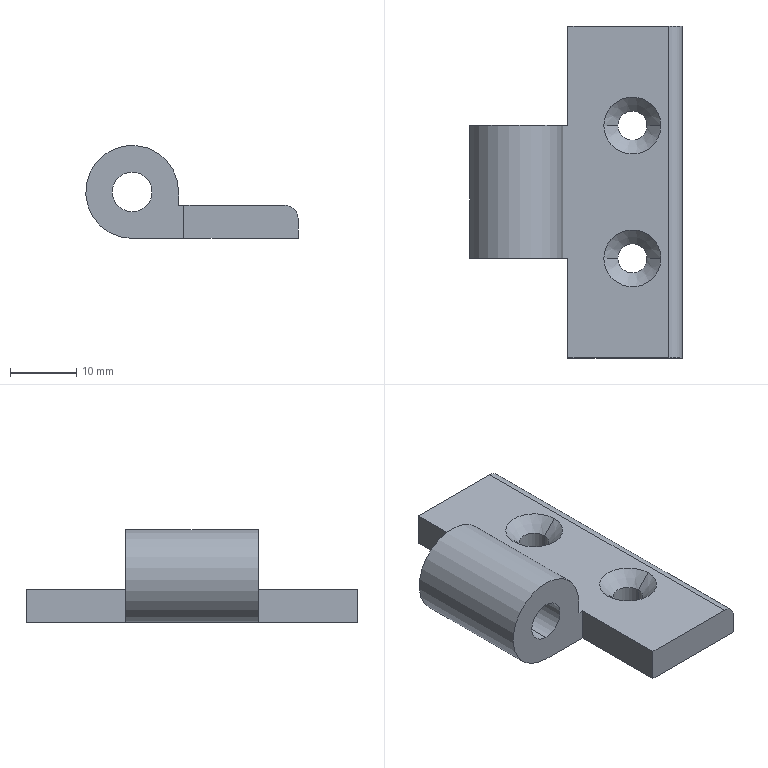Part | SolidWorks | features BaseBody 1 | 1 solid | 22 faces | box 32 x 50 x 14 mm | volume 6828 mm3 | plane 10 | cylinder 8 | cone 4 | commonest cylinder face diameters 4.4 x4 6 x2 4 x1 14 x1
STEP:
#1=CARTESIAN_POINT('',(0.,10.,4.));
#2=VERTEX_POINT('',#1);
#3=CARTESIAN_POINT('',(0.,10.,10.));
#4=VERTEX_POINT('',#3);
#5=CARTESIAN_POINT('',(0.,10.,7.));
#6=DIRECTION('',(0.,-1.,0.));
#7=DIRECTION('',(0.,0.,1.));
#8=AXIS2_PLACEMENT_3D('',#5,#6,#7);
#9=CIRCLE('',#8,3.);
#10=EDGE_CURVE('',#2,#4,#9,.T.);
#11=ORIENTED_EDGE('',*,*,#10,.F.);
#12=CARTESIAN_POINT('',(0.,-10.,4.));
#13=VERTEX_POINT('',#12);
#14=CARTESIAN_POINT('',(0.,23.,4.));
#15=DIRECTION('',(0.,-1.,0.));
#16=VECTOR('',#15,1000.);
#17=LINE('',#14,#16);
#18=EDGE_CURVE('',#2,#13,#17,.T.);
#19=ORIENTED_EDGE('',*,*,#18,.T.);
#20=CARTESIAN_POINT('',(0.,-10.,10.));
#21=VERTEX_POINT('',#20);
#22=CARTESIAN_POINT('',(0.,-10.,7.));
#23=DIRECTION('',(0.,1.,0.));
#24=DIRECTION('',(0.,0.,-1.));
#25=AXIS2_PLACEMENT_3D('',#22,#23,#24);
#26=CIRCLE('',#25,3.);
#27=EDGE_CURVE('',#21,#13,#26,.T.);
#28=ORIENTED_EDGE('',*,*,#27,.F.);
#29=CARTESIAN_POINT('',(0.,23.,10.));
#30=DIRECTION('',(0.,-1.,0.));
#31=VECTOR('',#30,1000.);
#32=LINE('',#29,#31);
#33=EDGE_CURVE('',#4,#21,#32,.T.);
#34=ORIENTED_EDGE('',*,*,#33,.F.);
#35=EDGE_LOOP('',(#11,#19,#28,#34));
#36=FACE_OUTER_BOUND('',#35,.T.);
#37=CARTESIAN_POINT('',(0.,23.,7.));
#38=DIRECTION('',(0.,-1.,0.));
#39=DIRECTION('',(0.,0.,1.));
#40=AXIS2_PLACEMENT_3D('',#37,#38,#39);
#41=CYLINDRICAL_SURFACE('',#40,3.);
#42=ADVANCED_FACE('',(#36),#41,.F.);
#43=CARTESIAN_POINT('',(15.3,-10.,0.));
#44=VERTEX_POINT('',#43);
#45=CARTESIAN_POINT('',(19.7,-10.,0.));
#46=VERTEX_POINT('',#45);
#47=CARTESIAN_POINT('',(17.5,-10.,0.));
#48=DIRECTION('',(0.,0.,-1.));
#49=DIRECTION('',(-1.,0.,0.));
#50=AXIS2_PLACEMENT_3D('',#47,#48,#49);
#51=CIRCLE('',#50,2.2);
#52=EDGE_CURVE('',#44,#46,#51,.T.);
#53=ORIENTED_EDGE('',*,*,#52,.T.);
#54=CARTESIAN_POINT('',(19.7,-10.,2.9));
#55=VERTEX_POINT('',#54);
#56=CARTESIAN_POINT('',(19.7,-10.,0.));
#57=DIRECTION('',(0.,0.,1.));
#58=VECTOR('',#57,1000.);
#59=LINE('',#56,#58);
#60=EDGE_CURVE('',#46,#55,#59,.T.);
#61=ORIENTED_EDGE('',*,*,#60,.T.);
#62=CARTESIAN_POINT('',(15.3,-10.,2.9));
#63=VERTEX_POINT('',#62);
#64=CARTESIAN_POINT('',(17.5,-10.,2.9));
#65=DIRECTION('',(0.,0.,-1.));
#66=DIRECTION('',(-1.,0.,0.));
#67=AXIS2_PLACEMENT_3D('',#64,#65,#66);
#68=CIRCLE('',#67,2.2);
#69=EDGE_CURVE('',#63,#55,#68,.T.);
#70=ORIENTED_EDGE('',*,*,#69,.F.);
#71=CARTESIAN_POINT('',(15.3,-10.,0.));
#72=DIRECTION('',(0.,0.,1.));
#73=VECTOR('',#72,1000.);
#74=LINE('',#71,#73);
#75=EDGE_CURVE('',#44,#63,#74,.T.);
#76=ORIENTED_EDGE('',*,*,#75,.F.);
#77=EDGE_LOOP('',(#53,#61,#70,#76));
#78=FACE_OUTER_BOUND('',#77,.T.);
#79=CARTESIAN_POINT('',(17.5,-10.,0.));
#80=DIRECTION('',(0.,0.,1.));
#81=DIRECTION('',(-1.,0.,0.));
#82=AXIS2_PLACEMENT_3D('',#79,#80,#81);
#83=CYLINDRICAL_SURFACE('',#82,2.2);
#84=ADVANCED_FACE('',(#78),#83,.F.);
#85=CARTESIAN_POINT('',(17.5,-10.,2.9));
#86=DIRECTION('',(0.,0.,-1.));
#87=DIRECTION('',(-1.,0.,0.));
#88=AXIS2_PLACEMENT_3D('',#85,#86,#87);
#89=CIRCLE('',#88,2.2);
#90=EDGE_CURVE('',#55,#63,#89,.T.);
#91=ORIENTED_EDGE('',*,*,#90,.T.);
#92=CARTESIAN_POINT('',(13.2,-10.,5.));
#93=VERTEX_POINT('',#92);
#94=CARTESIAN_POINT('',(13.2,-10.,5.));
#95=DIRECTION('',(-0.7071,0.,0.7071));
#96=VECTOR('',#95,1000.);
#97=LINE('',#94,#96);
#98=EDGE_CURVE('',#63,#93,#97,.T.);
#99=ORIENTED_EDGE('',*,*,#98,.T.);
#100=CARTESIAN_POINT('',(21.8,-10.,5.));
#101=VERTEX_POINT('',#100);
#102=CARTESIAN_POINT('',(17.5,-10.,5.));
#103=DIRECTION('',(0.,0.,-1.));
#104=DIRECTION('',(-1.,0.,0.));
#105=AXIS2_PLACEMENT_3D('',#102,#103,#104);
#106=CIRCLE('',#105,4.3);
#107=EDGE_CURVE('',#101,#93,#106,.T.);
#108=ORIENTED_EDGE('',*,*,#107,.F.);
#109=CARTESIAN_POINT('',(21.8,-10.,5.));
#110=DIRECTION('',(0.7071,0.,0.7071));
#111=VECTOR('',#110,1000.);
#112=LINE('',#109,#111);
#113=EDGE_CURVE('',#55,#101,#112,.T.);
#114=ORIENTED_EDGE('',*,*,#113,.F.);
#115=EDGE_LOOP('',(#91,#99,#108,#114));
#116=FACE_OUTER_BOUND('',#115,.T.);
#117=CARTESIAN_POINT('',(17.5,-10.,5.));
#118=DIRECTION('',(0.,0.,1.));
#119=DIRECTION('',(1.,0.,0.));
#120=AXIS2_PLACEMENT_3D('',#117,#118,#119);
#121=CONICAL_SURFACE('',#120,4.3,0.7854);
#122=ADVANCED_FACE('',(#116),#121,.F.);
#123=CARTESIAN_POINT('',(15.3,10.,0.));
#124=VERTEX_POINT('',#123);
#125=CARTESIAN_POINT('',(19.7,10.,0.));
#126=VERTEX_POINT('',#125);
#127=CARTESIAN_POINT('',(17.5,10.,0.));
#128=DIRECTION('',(0.,0.,-1.));
#129=DIRECTION('',(-1.,0.,0.));
#130=AXIS2_PLACEMENT_3D('',#127,#128,#129);
#131=CIRCLE('',#130,2.2);
#132=EDGE_CURVE('',#124,#126,#131,.T.);
#133=ORIENTED_EDGE('',*,*,#132,.T.);
#134=CARTESIAN_POINT('',(19.7,10.,2.9));
#135=VERTEX_POINT('',#134);
#136=CARTESIAN_POINT('',(19.7,10.,0.));
#137=DIRECTION('',(0.,0.,1.));
#138=VECTOR('',#137,1000.);
#139=LINE('',#136,#138);
#140=EDGE_CURVE('',#126,#135,#139,.T.);
#141=ORIENTED_EDGE('',*,*,#140,.T.);
#142=CARTESIAN_POINT('',(15.3,10.,2.9));
#143=VERTEX_POINT('',#142);
#144=CARTESIAN_POINT('',(17.5,10.,2.9));
#145=DIRECTION('',(0.,0.,-1.));
#146=DIRECTION('',(-1.,0.,0.));
#147=AXIS2_PLACEMENT_3D('',#144,#145,#146);
#148=CIRCLE('',#147,2.2);
#149=EDGE_CURVE('',#143,#135,#148,.T.);
#150=ORIENTED_EDGE('',*,*,#149,.F.);
#151=CARTESIAN_POINT('',(15.3,10.,0.));
#152=DIRECTION('',(0.,0.,1.));
#153=VECTOR('',#152,1000.);
#154=LINE('',#151,#153);
#155=EDGE_CURVE('',#124,#143,#154,.T.);
#156=ORIENTED_EDGE('',*,*,#155,.F.);
#157=EDGE_LOOP('',(#133,#141,#150,#156));
#158=FACE_OUTER_BOUND('',#157,.T.);
#159=CARTESIAN_POINT('',(17.5,10.,0.));
#160=DIRECTION('',(0.,0.,1.));
#161=DIRECTION('',(-1.,0.,0.));
#162=AXIS2_PLACEMENT_3D('',#159,#160,#161);
#163=CYLINDRICAL_SURFACE('',#162,2.2);
#164=ADVANCED_FACE('',(#158),#163,.F.);
#165=CARTESIAN_POINT('',(17.5,10.,2.9));
#166=DIRECTION('',(0.,0.,-1.));
#167=DIRECTION('',(-1.,0.,0.));
#168=AXIS2_PLACEMENT_3D('',#165,#166,#167);
#169=CIRCLE('',#168,2.2);
#170=EDGE_CURVE('',#135,#143,#169,.T.);
#171=ORIENTED_EDGE('',*,*,#170,.T.);
#172=CARTESIAN_POINT('',(13.2,10.,5.));
#173=VERTEX_POINT('',#172);
#174=CARTESIAN_POINT('',(13.2,10.,5.));
#175=DIRECTION('',(-0.7071,0.,0.7071));
#176=VECTOR('',#175,1000.);
#177=LINE('',#174,#176);
#178=EDGE_CURVE('',#143,#173,#177,.T.);
#179=ORIENTED_EDGE('',*,*,#178,.T.);
#180=CARTESIAN_POINT('',(21.8,10.,5.));
#181=VERTEX_POINT('',#180);
#182=CARTESIAN_POINT('',(17.5,10.,5.));
#183=DIRECTION('',(0.,0.,-1.));
#184=DIRECTION('',(-1.,0.,0.));
#185=AXIS2_PLACEMENT_3D('',#182,#183,#184);
#186=CIRCLE('',#185,4.3);
#187=EDGE_CURVE('',#181,#173,#186,.T.);
#188=ORIENTED_EDGE('',*,*,#187,.F.);
#189=CARTESIAN_POINT('',(21.8,10.,5.));
#190=DIRECTION('',(0.7071,0.,0.7071));
#191=VECTOR('',#190,1000.);
#192=LINE('',#189,#191);
#193=EDGE_CURVE('',#135,#181,#192,.T.);
#194=ORIENTED_EDGE('',*,*,#193,.F.);
#195=EDGE_LOOP('',(#171,#179,#188,#194));
#196=FACE_OUTER_BOUND('',#195,.T.);
#197=CARTESIAN_POINT('',(17.5,10.,5.));
#198=DIRECTION('',(0.,0.,1.));
#199=DIRECTION('',(1.,0.,0.));
#200=AXIS2_PLACEMENT_3D('',#197,#198,#199);
#201=CONICAL_SURFACE('',#200,4.3,0.7854);
#202=ADVANCED_FACE('',(#196),#201,.F.);
#203=CARTESIAN_POINT('',(7.,-10.,7.));
#204=VERTEX_POINT('',#203);
#205=CARTESIAN_POINT('',(0.,-10.,0.));
#206=VERTEX_POINT('',#205);
#207=CARTESIAN_POINT('',(0.,-10.,7.));
#208=DIRECTION('',(0.,-1.,0.));
#209=DIRECTION('',(0.,0.,-1.));
#210=AXIS2_PLACEMENT_3D('',#207,#208,#209);
#211=CIRCLE('',#210,7.);
#212=EDGE_CURVE('',#204,#206,#211,.T.);
#213=ORIENTED_EDGE('',*,*,#212,.F.);
#214=CARTESIAN_POINT('',(7.,10.,7.));
#215=VERTEX_POINT('',#214);
#216=CARTESIAN_POINT('',(7.,25.,7.));
#217=DIRECTION('',(0.,-1.,0.));
#218=VECTOR('',#217,1000.);
#219=LINE('',#216,#218);
#220=EDGE_CURVE('',#215,#204,#219,.T.);
#221=ORIENTED_EDGE('',*,*,#220,.F.);
#222=CARTESIAN_POINT('',(0.,10.,0.));
#223=VERTEX_POINT('',#222);
#224=CARTESIAN_POINT('',(0.,10.,7.));
#225=DIRECTION('',(0.,1.,0.));
#226=DIRECTION('',(0.,0.,1.));
#227=AXIS2_PLACEMENT_3D('',#224,#225,#226);
#228=CIRCLE('',#227,7.);
#229=EDGE_CURVE('',#223,#215,#228,.T.);
#230=ORIENTED_EDGE('',*,*,#229,.F.);
#231=CARTESIAN_POINT('',(0.,25.,0.));
#232=DIRECTION('',(0.,-1.,0.));
#233=VECTOR('',#232,1000.);
#234=LINE('',#231,#233);
#235=EDGE_CURVE('',#223,#206,#234,.T.);
#236=ORIENTED_EDGE('',*,*,#235,.T.);
#237=EDGE_LOOP('',(#213,#221,#230,#236));
#238=FACE_OUTER_BOUND('',#237,.T.);
#239=CARTESIAN_POINT('',(0.,25.,7.));
#240=DIRECTION('',(0.,1.,0.));
#241=DIRECTION('',(0.,0.,-1.));
#242=AXIS2_PLACEMENT_3D('',#239,#240,#241);
#243=CYLINDRICAL_SURFACE('',#242,7.);
#244=ADVANCED_FACE('',(#238),#243,.T.);
#245=CARTESIAN_POINT('',(7.,-10.,5.));
#246=VERTEX_POINT('',#245);
#247=CARTESIAN_POINT('',(7.,-10.,7.));
#248=DIRECTION('',(0.,0.,1.));
#249=VECTOR('',#248,1000.);
#250=LINE('',#247,#249);
#251=EDGE_CURVE('',#246,#204,#250,.T.);
#252=ORIENTED_EDGE('',*,*,#251,.F.);
#253=CARTESIAN_POINT('',(7.,10.,5.));
#254=VERTEX_POINT('',#253);
#255=CARTESIAN_POINT('',(7.,25.,5.));
#256=DIRECTION('',(0.,-1.,0.));
#257=VECTOR('',#256,1000.);
#258=LINE('',#255,#257);
#259=EDGE_CURVE('',#254,#246,#258,.T.);
#260=ORIENTED_EDGE('',*,*,#259,.F.);
#261=CARTESIAN_POINT('',(7.,10.,7.));
#262=DIRECTION('',(0.,0.,-1.));
#263=VECTOR('',#262,1000.);
#264=LINE('',#261,#263);
#265=EDGE_CURVE('',#215,#254,#264,.T.);
#266=ORIENTED_EDGE('',*,*,#265,.F.);
#267=ORIENTED_EDGE('',*,*,#220,.T.);
#268=EDGE_LOOP('',(#252,#260,#266,#267));
#269=FACE_OUTER_BOUND('',#268,.T.);
#270=CARTESIAN_POINT('',(7.,25.,7.));
#271=DIRECTION('',(-1.,0.,0.));
#272=DIRECTION('',(0.,0.,1.));
#273=AXIS2_PLACEMENT_3D('',#270,#271,#272);
#274=PLANE('',#273);
#275=ADVANCED_FACE('',(#269),#274,.F.);
#276=CARTESIAN_POINT('',(7.8,-25.,0.));
#277=VERTEX_POINT('',#276);
#278=CARTESIAN_POINT('',(7.8,-10.,0.));
#279=VERTEX_POINT('',#278);
#280=CARTESIAN_POINT('',(7.8,-25.,0.));
#281=DIRECTION('',(0.,1.,0.));
#282=VECTOR('',#281,1000.);
#283=LINE('',#280,#282);
#284=EDGE_CURVE('',#277,#279,#283,.T.);
#285=ORIENTED_EDGE('',*,*,#284,.T.);
#286=CARTESIAN_POINT('',(7.8,-10.,0.));
#287=DIRECTION('',(-1.,0.,0.));
#288=VECTOR('',#287,1000.);
#289=LINE('',#286,#288);
#290=EDGE_CURVE('',#279,#206,#289,.T.);
#291=ORIENTED_EDGE('',*,*,#290,.T.);
#292=ORIENTED_EDGE('',*,*,#235,.F.);
#293=CARTESIAN_POINT('',(7.8,10.,0.));
#294=VERTEX_POINT('',#293);
#295=CARTESIAN_POINT('',(-14.,10.,0.));
#296=DIRECTION('',(1.,0.,0.));
#297=VECTOR('',#296,1000.);
#298=LINE('',#295,#297);
#299=EDGE_CURVE('',#223,#294,#298,.T.);
#300=ORIENTED_EDGE('',*,*,#299,.T.);
#301=CARTESIAN_POINT('',(7.8,25.,0.));
#302=VERTEX_POINT('',#301);
#303=CARTESIAN_POINT('',(7.8,10.,0.));
#304=DIRECTION('',(0.,1.,0.));
#305=VECTOR('',#304,1000.);
#306=LINE('',#303,#305);
#307=EDGE_CURVE('',#294,#302,#306,.T.);
#308=ORIENTED_EDGE('',*,*,#307,.T.);
#309=CARTESIAN_POINT('',(25.,25.,0.));
#310=VERTEX_POINT('',#309);
#311=CARTESIAN_POINT('',(25.,25.,0.));
#312=DIRECTION('',(-1.,0.,0.));
#313=VECTOR('',#312,1000.);
#314=LINE('',#311,#313);
#315=EDGE_CURVE('',#310,#302,#314,.T.);
#316=ORIENTED_EDGE('',*,*,#315,.F.);
#317=CARTESIAN_POINT('',(25.,-25.,0.));
#318=VERTEX_POINT('',#317);
#319=CARTESIAN_POINT('',(25.,25.,0.));
#320=DIRECTION('',(0.,-1.,0.));
#321=VECTOR('',#320,1000.);
#322=LINE('',#319,#321);
#323=EDGE_CURVE('',#310,#318,#322,.T.);
#324=ORIENTED_EDGE('',*,*,#323,.T.);
#325=CARTESIAN_POINT('',(25.,-25.,0.));
#326=DIRECTION('',(-1.,0.,0.));
#327=VECTOR('',#326,1000.);
#328=LINE('',#325,#327);
#329=EDGE_CURVE('',#318,#277,#328,.T.);
#330=ORIENTED_EDGE('',*,*,#329,.T.);
#331=EDGE_LOOP('',(#285,#291,#292,#300,#308,#316,#324,#330));
#332=FACE_OUTER_BOUND('',#331,.T.);
#333=ORIENTED_EDGE('',*,*,#52,.F.);
#334=CARTESIAN_POINT('',(17.5,-10.,0.));
#335=DIRECTION('',(0.,0.,-1.));
#336=DIRECTION('',(-1.,0.,0.));
#337=AXIS2_PLACEMENT_3D('',#334,#335,#336);
#338=CIRCLE('',#337,2.2);
#339=EDGE_CURVE('',#46,#44,#338,.T.);
#340=ORIENTED_EDGE('',*,*,#339,.F.);
#341=EDGE_LOOP('',(#333,#340));
#342=FACE_BOUND('',#341,.T.);
#343=ORIENTED_EDGE('',*,*,#132,.F.);
#344=CARTESIAN_POINT('',(17.5,10.,0.));
#345=DIRECTION('',(0.,0.,-1.));
#346=DIRECTION('',(-1.,0.,0.));
#347=AXIS2_PLACEMENT_3D('',#344,#345,#346);
#348=CIRCLE('',#347,2.2);
#349=EDGE_CURVE('',#126,#124,#348,.T.);
#350=ORIENTED_EDGE('',*,*,#349,.F.);
#351=EDGE_LOOP('',(#343,#350));
#352=FACE_BOUND('',#351,.T.);
#353=CARTESIAN_POINT('',(25.,25.,0.));
#354=DIRECTION('',(0.,0.,1.));
#355=DIRECTION('',(1.,0.,0.));
#356=AXIS2_PLACEMENT_3D('',#353,#354,#355);
#357=PLANE('',#356);
#358=ADVANCED_FACE('',(#332,#342,#352),#357,.F.);
#359=CARTESIAN_POINT('',(7.8,-25.,5.));
#360=VERTEX_POINT('',#359);
#361=CARTESIAN_POINT('',(7.8,-10.,5.));
#362=VERTEX_POINT('',#361);
#363=CARTESIAN_POINT('',(7.8,25.,5.));
#364=DIRECTION('',(0.,1.,0.));
#365=VECTOR('',#364,1000.);
#366=LINE('',#363,#365);
#367=EDGE_CURVE('',#360,#362,#366,.T.);
#368=ORIENTED_EDGE('',*,*,#367,.F.);
#369=CARTESIAN_POINT('',(23.,-25.,5.));
#370=VERTEX_POINT('',#369);
#371=CARTESIAN_POINT('',(7.,-25.,5.));
#372=DIRECTION('',(1.,0.,0.));
#373=VECTOR('',#372,1000.);
#374=LINE('',#371,#373);
#375=EDGE_CURVE('',#360,#370,#374,.T.);
#376=ORIENTED_EDGE('',*,*,#375,.T.);
#377=CARTESIAN_POINT('',(23.,25.,5.));
#378=VERTEX_POINT('',#377);
#379=CARTESIAN_POINT('',(23.,25.,5.));
#380=DIRECTION('',(0.,-1.,0.));
#381=VECTOR('',#380,1000.);
#382=LINE('',#379,#381);
#383=EDGE_CURVE('',#378,#370,#382,.T.);
#384=ORIENTED_EDGE('',*,*,#383,.F.);
#385=CARTESIAN_POINT('',(7.8,25.,5.));
#386=VERTEX_POINT('',#385);
#387=CARTESIAN_POINT('',(7.,25.,5.));
#388=DIRECTION('',(1.,0.,0.));
#389=VECTOR('',#388,1000.);
#390=LINE('',#387,#389);
#391=EDGE_CURVE('',#386,#378,#390,.T.);
#392=ORIENTED_EDGE('',*,*,#391,.F.);
#393=CARTESIAN_POINT('',(7.8,10.,5.));
#394=VERTEX_POINT('',#393);
#395=CARTESIAN_POINT('',(7.8,25.,5.));
#396=DIRECTION('',(0.,1.,0.));
#397=VECTOR('',#396,1000.);
#398=LINE('',#395,#397);
#399=EDGE_CURVE('',#394,#386,#398,.T.);
#400=ORIENTED_EDGE('',*,*,#399,.F.);
#401=CARTESIAN_POINT('',(7.,10.,5.));
#402=DIRECTION('',(1.,0.,0.));
#403=VECTOR('',#402,1000.);
#404=LINE('',#401,#403);
#405=EDGE_CURVE('',#254,#394,#404,.T.);
#406=ORIENTED_EDGE('',*,*,#405,.F.);
#407=ORIENTED_EDGE('',*,*,#259,.T.);
#408=CARTESIAN_POINT('',(7.,-10.,5.));
#409=DIRECTION('',(-1.,0.,0.));
#410=VECTOR('',#409,1000.);
#411=LINE('',#408,#410);
#412=EDGE_CURVE('',#362,#246,#411,.T.);
#413=ORIENTED_EDGE('',*,*,#412,.F.);
#414=EDGE_LOOP('',(#368,#376,#384,#392,#400,#406,#407,#413));
#415=FACE_OUTER_BOUND('',#414,.T.);
#416=ORIENTED_EDGE('',*,*,#107,.T.);
#417=CARTESIAN_POINT('',(17.5,-10.,5.));
#418=DIRECTION('',(0.,0.,-1.));
#419=DIRECTION('',(-1.,0.,0.));
#420=AXIS2_PLACEMENT_3D('',#417,#418,#419);
#421=CIRCLE('',#420,4.3);
#422=EDGE_CURVE('',#93,#101,#421,.T.);
#423=ORIENTED_EDGE('',*,*,#422,.T.);
#424=EDGE_LOOP('',(#416,#423));
#425=FACE_BOUND('',#424,.T.);
#426=ORIENTED_EDGE('',*,*,#187,.T.);
#427=CARTESIAN_POINT('',(17.5,10.,5.));
#428=DIRECTION('',(0.,0.,-1.));
#429=DIRECTION('',(-1.,0.,0.));
#430=AXIS2_PLACEMENT_3D('',#427,#428,#429);
#431=CIRCLE('',#430,4.3);
#432=EDGE_CURVE('',#173,#181,#431,.T.);
#433=ORIENTED_EDGE('',*,*,#432,.T.);
#434=EDGE_LOOP('',(#426,#433));
#435=FACE_BOUND('',#434,.T.);
#436=CARTESIAN_POINT('',(7.,25.,5.));
#437=DIRECTION('',(0.,0.,-1.));
#438=DIRECTION('',(0.,-1.,0.));
#439=AXIS2_PLACEMENT_3D('',#436,#437,#438);
#440=PLANE('',#439);
#441=ADVANCED_FACE('',(#415,#425,#435),#440,.F.);
#442=CARTESIAN_POINT('',(25.,-25.,3.));
#443=VERTEX_POINT('',#442);
#444=CARTESIAN_POINT('',(23.,-25.,3.));
#445=DIRECTION('',(0.,1.,0.));
#446=DIRECTION('',(1.,0.,0.));
#447=AXIS2_PLACEMENT_3D('',#444,#445,#446);
#448=CIRCLE('',#447,2.);
#449=EDGE_CURVE('',#370,#443,#448,.T.);
#450=ORIENTED_EDGE('',*,*,#449,.T.);
#451=CARTESIAN_POINT('',(25.,25.,3.));
#452=VERTEX_POINT('',#451);
#453=CARTESIAN_POINT('',(25.,25.,3.));
#454=DIRECTION('',(0.,-1.,0.));
#455=VECTOR('',#454,1000.);
#456=LINE('',#453,#455);
#457=EDGE_CURVE('',#452,#443,#456,.T.);
#458=ORIENTED_EDGE('',*,*,#457,.F.);
#459=CARTESIAN_POINT('',(23.,25.,3.));
#460=DIRECTION('',(0.,1.,0.));
#461=DIRECTION('',(1.,0.,0.));
#462=AXIS2_PLACEMENT_3D('',#459,#460,#461);
#463=CIRCLE('',#462,2.);
#464=EDGE_CURVE('',#378,#452,#463,.T.);
#465=ORIENTED_EDGE('',*,*,#464,.F.);
#466=ORIENTED_EDGE('',*,*,#383,.T.);
#467=EDGE_LOOP('',(#450,#458,#465,#466));
#468=FACE_OUTER_BOUND('',#467,.T.);
#469=CARTESIAN_POINT('',(23.,25.,3.));
#470=DIRECTION('',(0.,1.,0.));
#471=DIRECTION('',(0.,0.,-1.));
#472=AXIS2_PLACEMENT_3D('',#469,#470,#471);
#473=CYLINDRICAL_SURFACE('',#472,2.);
#474=ADVANCED_FACE('',(#468),#473,.T.);
#475=CARTESIAN_POINT('',(25.,-25.,3.));
#476=DIRECTION('',(0.,0.,-1.));
#477=VECTOR('',#476,1000.);
#478=LINE('',#475,#477);
#479=EDGE_CURVE('',#443,#318,#478,.T.);
#480=ORIENTED_EDGE('',*,*,#479,.T.);
#481=ORIENTED_EDGE('',*,*,#323,.F.);
#482=CARTESIAN_POINT('',(25.,25.,3.));
#483=DIRECTION('',(0.,0.,-1.));
#484=VECTOR('',#483,1000.);
#485=LINE('',#482,#484);
#486=EDGE_CURVE('',#452,#310,#485,.T.);
#487=ORIENTED_EDGE('',*,*,#486,.F.);
#488=ORIENTED_EDGE('',*,*,#457,.T.);
#489=EDGE_LOOP('',(#480,#481,#487,#488));
#490=FACE_OUTER_BOUND('',#489,.T.);
#491=CARTESIAN_POINT('',(25.,25.,3.));
#492=DIRECTION('',(-1.,0.,0.));
#493=DIRECTION('',(0.,0.,1.));
#494=AXIS2_PLACEMENT_3D('',#491,#492,#493);
#495=PLANE('',#494);
#496=ADVANCED_FACE('',(#490),#495,.F.);
#497=CARTESIAN_POINT('',(7.8,-25.,14.));
#498=DIRECTION('',(0.,0.,-1.));
#499=VECTOR('',#498,1000.);
#500=LINE('',#497,#499);
#501=EDGE_CURVE('',#360,#277,#500,.T.);
#502=ORIENTED_EDGE('',*,*,#501,.T.);
#503=ORIENTED_EDGE('',*,*,#329,.F.);
#504=ORIENTED_EDGE('',*,*,#479,.F.);
#505=ORIENTED_EDGE('',*,*,#449,.F.);
#506=ORIENTED_EDGE('',*,*,#375,.F.);
#507=EDGE_LOOP('',(#502,#503,#504,#505,#506));
#508=FACE_OUTER_BOUND('',#507,.T.);
#509=CARTESIAN_POINT('',(0.,-25.,7.));
#510=DIRECTION('',(0.,1.,0.));
#511=DIRECTION('',(1.,0.,0.));
#512=AXIS2_PLACEMENT_3D('',#509,#510,#511);
#513=PLANE('',#512);
#514=ADVANCED_FACE('',(#508),#513,.F.);
#515=ORIENTED_EDGE('',*,*,#315,.T.);
#516=CARTESIAN_POINT('',(7.8,25.,14.));
#517=DIRECTION('',(0.,0.,-1.));
#518=VECTOR('',#517,1000.);
#519=LINE('',#516,#518);
#520=EDGE_CURVE('',#386,#302,#519,.T.);
#521=ORIENTED_EDGE('',*,*,#520,.F.);
#522=ORIENTED_EDGE('',*,*,#391,.T.);
#523=ORIENTED_EDGE('',*,*,#464,.T.);
#524=ORIENTED_EDGE('',*,*,#486,.T.);
#525=EDGE_LOOP('',(#515,#521,#522,#523,#524));
#526=FACE_OUTER_BOUND('',#525,.T.);
#527=CARTESIAN_POINT('',(0.,25.,7.));
#528=DIRECTION('',(0.,1.,0.));
#529=DIRECTION('',(1.,0.,0.));
#530=AXIS2_PLACEMENT_3D('',#527,#528,#529);
#531=PLANE('',#530);
#532=ADVANCED_FACE('',(#526),#531,.T.);
#533=ORIENTED_EDGE('',*,*,#367,.T.);
#534=CARTESIAN_POINT('',(7.8,-10.,14.));
#535=DIRECTION('',(0.,0.,-1.));
#536=VECTOR('',#535,1000.);
#537=LINE('',#534,#536);
#538=EDGE_CURVE('',#362,#279,#537,.T.);
#539=ORIENTED_EDGE('',*,*,#538,.T.);
#540=ORIENTED_EDGE('',*,*,#284,.F.);
#541=ORIENTED_EDGE('',*,*,#501,.F.);
#542=EDGE_LOOP('',(#533,#539,#540,#541));
#543=FACE_OUTER_BOUND('',#542,.T.);
#544=CARTESIAN_POINT('',(7.8,-25.,14.));
#545=DIRECTION('',(-1.,0.,0.));
#546=DIRECTION('',(0.,0.,1.));
#547=AXIS2_PLACEMENT_3D('',#544,#545,#546);
#548=PLANE('',#547);
#549=ADVANCED_FACE('',(#543),#548,.T.);
#550=ORIENTED_EDGE('',*,*,#212,.T.);
#551=ORIENTED_EDGE('',*,*,#290,.F.);
#552=ORIENTED_EDGE('',*,*,#538,.F.);
#553=ORIENTED_EDGE('',*,*,#412,.T.);
#554=ORIENTED_EDGE('',*,*,#251,.T.);
#555=EDGE_LOOP('',(#550,#551,#552,#553,#554));
#556=FACE_OUTER_BOUND('',#555,.T.);
#557=ORIENTED_EDGE('',*,*,#27,.T.);
#558=CARTESIAN_POINT('',(0.,-10.,7.));
#559=DIRECTION('',(0.,1.,0.));
#560=DIRECTION('',(0.,0.,-1.));
#561=AXIS2_PLACEMENT_3D('',#558,#559,#560);
#562=CIRCLE('',#561,3.);
#563=EDGE_CURVE('',#13,#21,#562,.T.);
#564=ORIENTED_EDGE('',*,*,#563,.T.);
#565=EDGE_LOOP('',(#557,#564));
#566=FACE_BOUND('',#565,.T.);
#567=CARTESIAN_POINT('',(7.8,-10.,14.));
#568=DIRECTION('',(0.,-1.,0.));
#569=DIRECTION('',(0.,0.,-1.));
#570=AXIS2_PLACEMENT_3D('',#567,#568,#569);
#571=PLANE('',#570);
#572=ADVANCED_FACE('',(#556,#566),#571,.T.);
#573=ORIENTED_EDGE('',*,*,#229,.T.);
#574=ORIENTED_EDGE('',*,*,#265,.T.);
#575=ORIENTED_EDGE('',*,*,#405,.T.);
#576=CARTESIAN_POINT('',(7.8,10.,14.));
#577=DIRECTION('',(0.,0.,-1.));
#578=VECTOR('',#577,1000.);
#579=LINE('',#576,#578);
#580=EDGE_CURVE('',#394,#294,#579,.T.);
#581=ORIENTED_EDGE('',*,*,#580,.T.);
#582=ORIENTED_EDGE('',*,*,#299,.F.);
#583=EDGE_LOOP('',(#573,#574,#575,#581,#582));
#584=FACE_OUTER_BOUND('',#583,.T.);
#585=CARTESIAN_POINT('',(0.,10.,7.));
#586=DIRECTION('',(0.,-1.,0.));
#587=DIRECTION('',(0.,0.,1.));
#588=AXIS2_PLACEMENT_3D('',#585,#586,#587);
#589=CIRCLE('',#588,3.);
#590=EDGE_CURVE('',#4,#2,#589,.T.);
#591=ORIENTED_EDGE('',*,*,#590,.T.);
#592=ORIENTED_EDGE('',*,*,#10,.T.);
#593=EDGE_LOOP('',(#591,#592));
#594=FACE_BOUND('',#593,.T.);
#595=CARTESIAN_POINT('',(-14.,10.,14.));
#596=DIRECTION('',(0.,1.,0.));
#597=DIRECTION('',(1.,0.,0.));
#598=AXIS2_PLACEMENT_3D('',#595,#596,#597);
#599=PLANE('',#598);
#600=ADVANCED_FACE('',(#584,#594),#599,.T.);
#601=ORIENTED_EDGE('',*,*,#399,.T.);
#602=ORIENTED_EDGE('',*,*,#520,.T.);
#603=ORIENTED_EDGE('',*,*,#307,.F.);
#604=ORIENTED_EDGE('',*,*,#580,.F.);
#605=EDGE_LOOP('',(#601,#602,#603,#604));
#606=FACE_OUTER_BOUND('',#605,.T.);
#607=CARTESIAN_POINT('',(7.8,10.,14.));
#608=DIRECTION('',(-1.,0.,0.));
#609=DIRECTION('',(0.,0.,1.));
#610=AXIS2_PLACEMENT_3D('',#607,#608,#609);
#611=PLANE('',#610);
#612=ADVANCED_FACE('',(#606),#611,.T.);
#613=ORIENTED_EDGE('',*,*,#178,.F.);
#614=ORIENTED_EDGE('',*,*,#149,.T.);
#615=ORIENTED_EDGE('',*,*,#193,.T.);
#616=ORIENTED_EDGE('',*,*,#432,.F.);
#617=EDGE_LOOP('',(#613,#614,#615,#616));
#618=FACE_OUTER_BOUND('',#617,.T.);
#619=CARTESIAN_POINT('',(17.5,10.,5.));
#620=DIRECTION('',(0.,0.,1.));
#621=DIRECTION('',(1.,0.,0.));
#622=AXIS2_PLACEMENT_3D('',#619,#620,#621);
#623=CONICAL_SURFACE('',#622,4.3,0.7854);
#624=ADVANCED_FACE('',(#618),#623,.F.);
#625=ORIENTED_EDGE('',*,*,#140,.F.);
#626=ORIENTED_EDGE('',*,*,#349,.T.);
#627=ORIENTED_EDGE('',*,*,#155,.T.);
#628=ORIENTED_EDGE('',*,*,#170,.F.);
#629=EDGE_LOOP('',(#625,#626,#627,#628));
#630=FACE_OUTER_BOUND('',#629,.T.);
#631=CARTESIAN_POINT('',(17.5,10.,0.));
#632=DIRECTION('',(0.,0.,1.));
#633=DIRECTION('',(-1.,0.,0.));
#634=AXIS2_PLACEMENT_3D('',#631,#632,#633);
#635=CYLINDRICAL_SURFACE('',#634,2.2);
#636=ADVANCED_FACE('',(#630),#635,.F.);
#637=ORIENTED_EDGE('',*,*,#98,.F.);
#638=ORIENTED_EDGE('',*,*,#69,.T.);
#639=ORIENTED_EDGE('',*,*,#113,.T.);
#640=ORIENTED_EDGE('',*,*,#422,.F.);
#641=EDGE_LOOP('',(#637,#638,#639,#640));
#642=FACE_OUTER_BOUND('',#641,.T.);
#643=CARTESIAN_POINT('',(17.5,-10.,5.));
#644=DIRECTION('',(0.,0.,1.));
#645=DIRECTION('',(1.,0.,0.));
#646=AXIS2_PLACEMENT_3D('',#643,#644,#645);
#647=CONICAL_SURFACE('',#646,4.3,0.7854);
#648=ADVANCED_FACE('',(#642),#647,.F.);
#649=ORIENTED_EDGE('',*,*,#60,.F.);
#650=ORIENTED_EDGE('',*,*,#339,.T.);
#651=ORIENTED_EDGE('',*,*,#75,.T.);
#652=ORIENTED_EDGE('',*,*,#90,.F.);
#653=EDGE_LOOP('',(#649,#650,#651,#652));
#654=FACE_OUTER_BOUND('',#653,.T.);
#655=CARTESIAN_POINT('',(17.5,-10.,0.));
#656=DIRECTION('',(0.,0.,1.));
#657=DIRECTION('',(-1.,0.,0.));
#658=AXIS2_PLACEMENT_3D('',#655,#656,#657);
#659=CYLINDRICAL_SURFACE('',#658,2.2);
#660=ADVANCED_FACE('',(#654),#659,.F.);
#661=ORIENTED_EDGE('',*,*,#18,.F.);
#662=ORIENTED_EDGE('',*,*,#590,.F.);
#663=ORIENTED_EDGE('',*,*,#33,.T.);
#664=ORIENTED_EDGE('',*,*,#563,.F.);
#665=EDGE_LOOP('',(#661,#662,#663,#664));
#666=FACE_OUTER_BOUND('',#665,.T.);
#667=CARTESIAN_POINT('',(0.,23.,7.));
#668=DIRECTION('',(0.,-1.,0.));
#669=DIRECTION('',(0.,0.,1.));
#670=AXIS2_PLACEMENT_3D('',#667,#668,#669);
#671=CYLINDRICAL_SURFACE('',#670,3.);
#672=ADVANCED_FACE('',(#666),#671,.F.);
#673=CLOSED_SHELL('',(#42,#84,#122,#164,#202,#244,#275,#358,#441,#474,#496,#514,#532,#549,#572,#600,#612,#624,#636,#648,#660,#672));
#674=MANIFOLD_SOLID_BREP('',#673);
#675=CARTESIAN_POINT('',(0.,0.,0.));
#676=DIRECTION('',(0.,0.,1.));
#677=DIRECTION('',(1.,0.,0.));
#678=AXIS2_PLACEMENT_3D('',#675,#676,#677);
#679=(LENGTH_UNIT()NAMED_UNIT(*)SI_UNIT(.MILLI.,.METRE.));
#680=UNCERTAINTY_MEASURE_WITH_UNIT(LENGTH_MEASURE(0.00001),#679,'','');
#681=(NAMED_UNIT(*)PLANE_ANGLE_UNIT()SI_UNIT($,.RADIAN.));
#682=(NAMED_UNIT(*)SI_UNIT($,.STERADIAN.)SOLID_ANGLE_UNIT());
#683=(GEOMETRIC_REPRESENTATION_CONTEXT(3)GLOBAL_UNCERTAINTY_ASSIGNED_CONTEXT((#680))GLOBAL_UNIT_ASSIGNED_CONTEXT((#679,#681,#682))REPRESENTATION_CONTEXT('',''));
#684=ADVANCED_BREP_SHAPE_REPRESENTATION('',(#674,#678),#683);